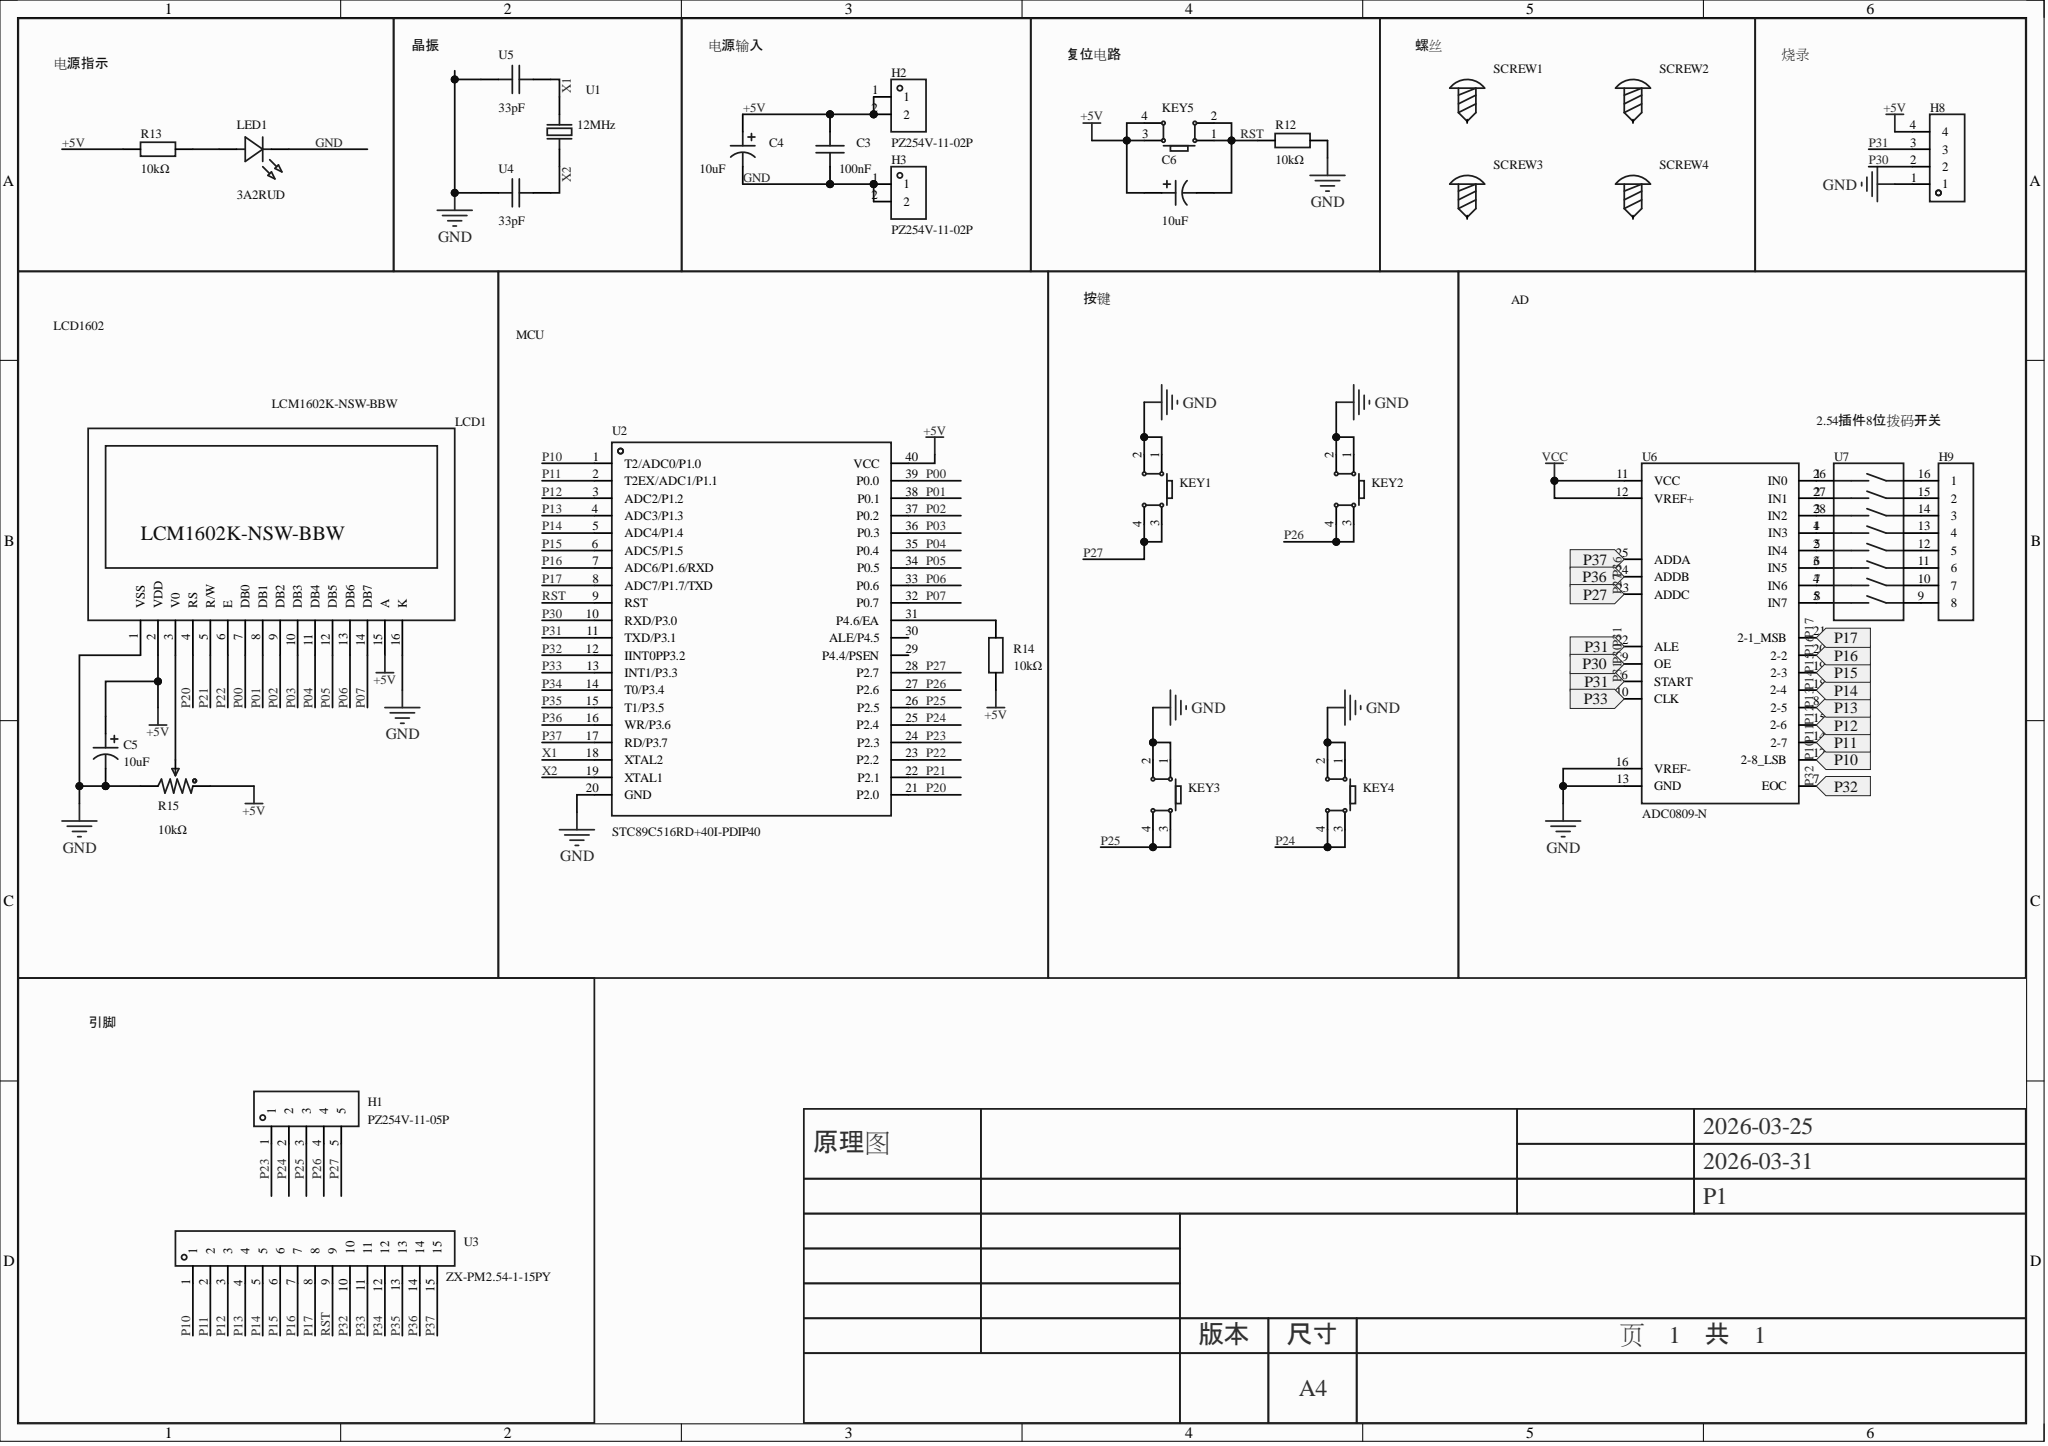Circuit board | Altium Designer | 31 parts | 57 nets
Bill of materials:
Comment,Description,Designator,Footprint,LibRef,Quantity
"100nF","","C3","CAP-TH_L5.0-W2.5-P5.00-D1.0","CC1H104MC1FD3F6C10MF","1"
"10uF","","C4, C5, C6","CAP-TH_BD5.0-P2.00-D0.5-FD-A","ERG50V10M5X11","3"
"PZ254V-11-05P","","H1","HDR-TH_5P-P2.54-V-M","PZ254V-11-05P","1"
"PZ254V-11-02P","","H2, H3","HDR-TH_2P-P2.54-V-M","PZ254V-11-02P","2"
"","","H8","HDR-TH_4P-P2.54-V-F","HDR-F_2.54_1x4P","1"
"","","H9","HDR-TH_8P-P2.54-V-F-1","HDR-F_2.54_1x8P","1"
"","","KEY1, KEY2, KEY3, KEY4, KEY5","SW-TH_4P-L6.0-W6.0-P4.50-LS6.5","Key_TH_6x6x6","5"
"LCM1602K-NSW-BBW","","LCD1","MODULE-TH_LCM1602K","LCM1602K-NSW-BBW","1"
"3A2RUD","","LED1","LED-TH_BD3.5-P2.28_3A2RUC","3A2RUD","1"
"10kΩ","","R12, R13, R14","RES-TH_BD2.3-L6.5-P10.50-D0.5","MF1/4W-10KΩ±1% T","3"
"10kΩ","","R15","RES-ADJ-TH_3P-L10.0-W10.0-P2.50-L","3296W-1-103","1"
"","","SCREW1, SCREW2, SCREW3, SCREW4","M3螺丝","M3螺丝","4"
"12MHz","","U1","HC-49S_L11.0-W4.7-P4.88","YG12MLBBE2X","1"
"STC89C516RD+40I-PDIP40","","U2","DIP-40_L52.3-W13.9-P2.54-LS15.2-BL","STC89C516RD+40I-PDIP40","1"
"ZX-PM2.54-1-15PY","","U3","HDR-TH_15P-P2.54-V-F","ZX-PM2.54-1-15PY","1"
"33pF","","U4, U5","CAP-TH_L5.0-W2.5-P5.08-D0.7","CC1H330JC74DCH4B10MN","2"
"ADC0809-N","","U6","PDIP-28_L36.0-W13.0-P2.54-LS15.5-BL","ADC0809-N","1"
"2.54插件8位拨码开关","","U7","SW-TH_16P-L21.9-W9.9-P2.54-LS7.8","2.54插件8位拨码开关","1"
Netlist (Protel format):
[
C3
CAP-TH_L5.0-W2.5-P5.00-D1.0
100nF



]
[
C4
CAP-TH_BD5.0-P2.00-D0.5-FD-A
10uF



]
[
C5
CAP-TH_BD5.0-P2.00-D0.5-FD-A
10uF



]
[
C6
CAP-TH_BD5.0-P2.00-D0.5-FD-A
10uF



]
[
H1
HDR-TH_5P-P2.54-V-M
PZ254V-11-05P



]
[
H2
HDR-TH_2P-P2.54-V-M
PZ254V-11-02P



]
[
H3
HDR-TH_2P-P2.54-V-M
PZ254V-11-02P



]
[
H8
HDR-TH_4P-P2.54-V-F




]
[
H9
HDR-TH_8P-P2.54-V-F-1




]
[
KEY1
SW-TH_4P-L6.0-W6.0-P4.50-LS6.5




]
[
KEY2
SW-TH_4P-L6.0-W6.0-P4.50-LS6.5




]
[
KEY3
SW-TH_4P-L6.0-W6.0-P4.50-LS6.5




]
[
KEY4
SW-TH_4P-L6.0-W6.0-P4.50-LS6.5




]
[
KEY5
SW-TH_4P-L6.0-W6.0-P4.50-LS6.5




]
[
LCD1
MODULE-TH_LCM1602K
LCM1602K-NSW-BBW



]
[
LED1
LED-TH_BD3.5-P2.28_3A2RUC
3A2RUD



]
[
R12
RES-TH_BD2.3-L6.5-P10.50-D0.5
10kΩ



]
[
R13
RES-TH_BD2.3-L6.5-P10.50-D0.5
10kΩ



]
[
R14
RES-TH_BD2.3-L6.5-P10.50-D0.5
10kΩ



]
[
R15
RES-ADJ-TH_3P-L10.0-W10.0-P2.50-L
10kΩ



]
[
SCREW1
M3螺丝




]
[
SCREW2
M3螺丝




]
[
SCREW3
M3螺丝




]
[
SCREW4
M3螺丝




]
[
U1
HC-49S_L11.0-W4.7-P4.88
12MHz



]
[
U2
DIP-40_L52.3-W13.9-P2.54-LS15.2-BL
STC89C516RD+40I-PDIP40



]
[
U3
HDR-TH_15P-P2.54-V-F
ZX-PM2.54-1-15PY



]
[
U4
CAP-TH_L5.0-W2.5-P5.08-D0.7
33pF



]
[
U5
CAP-TH_L5.0-W2.5-P5.08-D0.7
33pF



]
[
U6
PDIP-28_L36.0-W13.0-P2.54-LS15.5-BL
ADC0809-N



]
[
U7
SW-TH_16P-L21.9-W9.9-P2.54-LS7.8
2.54插件8位拨码开关



]
(
X2
U1-1
U2-19
U4-2
)
(
X1
U1-2
U2-18
U5-2
)
(
VCC
U6-11
U6-12
)
(
RST
C6-2
KEY5-1
KEY5-2
R12-2
U2-9
U3-9
)
(
P37
U2-17
U3-15
)
(
P36
U2-16
U3-14
U6-24
)
(
P35
U2-15
U3-13
)
(
P34
U2-14
U3-12
)
(
P33
U2-13
U3-11
)
(
P32
U2-12
U3-10
U6-7
)
(
P31
H8-3
U2-11
U6-6
U6-22
)
(
P30
H8-2
U2-10
U6-9
)
(
P27
H1-5
KEY1-3
KEY1-4
U2-28
U6-23
)
(
P26
H1-4
KEY2-3
KEY2-4
U2-27
)
(
P25
H1-3
KEY3-3
KEY3-4
U2-26
)
(
P24
H1-2
KEY4-3
KEY4-4
U2-25
)
(
P23
H1-1
U2-24
)
(
P22
LCD1-6
U2-23
)
(
P21
LCD1-5
U2-22
)
(
P20
LCD1-4
U2-21
)
(
P17
U2-8
U3-8
U6-21
)
(
P16
U2-7
U3-7
U6-20
)
(
P15
U2-6
U3-6
U6-19
)
(
P14
U2-5
U3-5
U6-18
)
(
P13
U2-4
U3-4
U6-8
)
(
P12
U2-3
U3-3
U6-15
)
(
P11
U2-2
U3-2
U6-14
)
(
P10
U2-1
U3-1
U6-17
)
(
P07
LCD1-14
U2-32
)
(
P06
LCD1-13
U2-33
)
(
P05
LCD1-12
U2-34
)
(
P04
LCD1-11
U2-35
)
(
P03
LCD1-10
U2-36
)
(
P02
LCD1-9
U2-37
)
(
P01
LCD1-8
U2-38
)
(
P00
LCD1-7
U2-39
)
(
NetU6_28
U6-28
U7-3
)
(
NetU6_27
U6-27
U7-2
)
(
NetU6_26
U6-26
U7-1
)
(
NetU6_5
U6-5
U7-8
)
(
NetU6_4
U6-4
U7-7
)
(
NetU6_3
U6-3
U7-6
)
(
NetU6_2
U6-2
U7-5
)
(
NetU6_1
U6-1
U7-4
)
(
NetR14_2
R14-2
U2-31
)
(
NetLED1_2
LED1-2
R13-1
)
(
NetLCD1_3
LCD1-3
R15-2
)
(
NetH9_8
H9-8
U7-9
)
(
NetH9_7
H9-7
U7-10
)
(
NetH9_6
H9-6
U7-11
)
(
NetH9_5
H9-5
U7-12
)
(
NetH9_4
H9-4
U7-13
)
(
NetH9_3
H9-3
U7-14
)
(
NetH9_2
H9-2
U7-15
)
(
NetH9_1
H9-1
U7-16
)
(
GND
C3-1
C4-2
C5-2
H3-1
H3-2
H8-1
KEY1-1
KEY1-2
KEY2-1
KEY2-2
KEY3-1
KEY3-2
KEY4-1
KEY4-2
LCD1-1
LCD1-16
LED1-1
R12-1
R15-3
U2-20
U4-1
U5-1
U6-13
U6-16
)
(
+5V
C3-2
C4-1
C5-1
C6-1
H2-1
H2-2
H8-4
KEY5-3
KEY5-4
LCD1-2
LCD1-15
R13-2
R14-1
R15-1
U2-40
)